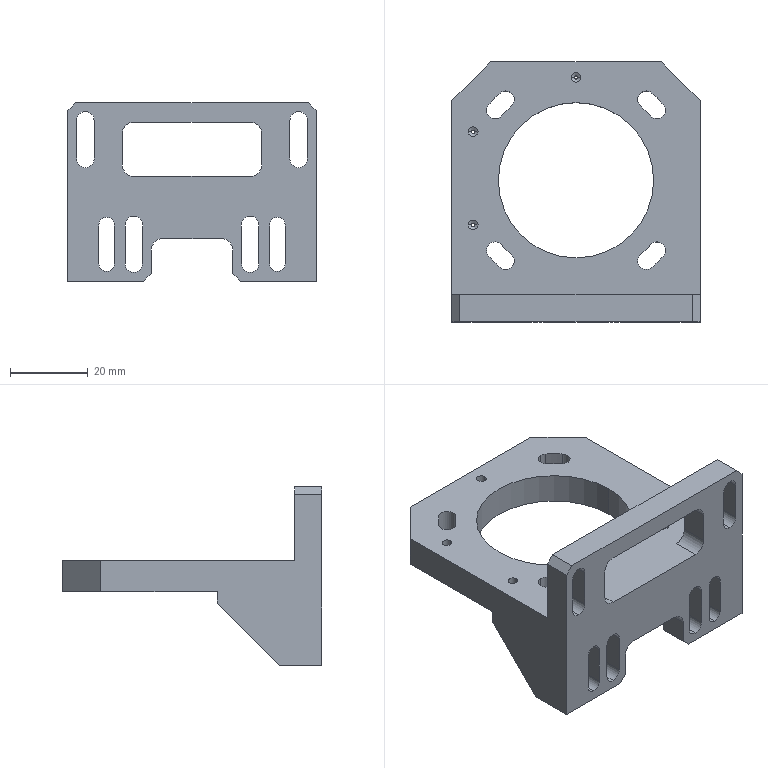NC program | NX | posted with a generic post | part box 64 x 67 x 46 mm
Lines 14041 to 14131 of 33790:
(DRILLING , TOOL : ZXZ)
N28068 T01 M6
N28070 G54
N28072 G17 G0 G90 X29.5 Y0. B0. C0. S3500 M3
N28074 G43 Z30. H1
N28076 G94 G81 G98 Z-20. F250. R-16.
N28078 X3.
N28080 X-8.5 Y26.5
N28082 X15.5
N28084 G80
N28086 G0 X15.5 Y26.5 Z30.
N28088 M5
(DRILLING_COPY , TOOL : 2.5ZT)
N28090 T12 M6
N28092 G54
N28094 G17 G0 G90 X29.5 Y0. B0. C0. S2000 M3
N28096 G43 Z30. H12
N28098 G94 G83 G98 Z-27.251 F120. Q2. R-16.
N28100 X15.5 Y26.5
N28102 X-8.5
N28104 G80
N28106 G0 X-8.5 Y26.5 Z30.
N28108 M5
(ZLEVEL_PROFILE_COPY , TOOL : D10JING)
N28110 T11 M6
N28112 G54
N28114 G17 G0 G90 X4.805 Y12.874 B0. C0. S5000 M3
N28116 G43 Z30. H11
N28118 Z-25.5
N28120 G94 G1 Z-27. F1000.
N28122 X3.866 Y14.5
N28124 G3 X3. Y15. R1.
N28126 X-12. Y0. R15. F1200.
N28128 X3. Y15. R-15.
N28130 X2.134 Y14.5 R1.
N28132 G1 X1.195 Y12.874
N28134 Z-25.5
N28136 G0 Z30.
(FLOOR_WALL_2 , TOOL : D10JING)
N28138 X34.03 Y29.956 S7000
N28140 Z-18.
N28142 G1 Z-19. F1250.
N28144 X33.999 Y29.938
N28146 G3 X33.499 Y29.072 R1.
N28148 G1 Y-29.072
N28150 X28.545 Y-34.027
N28152 Y34.027
N28154 X25.571 Y37.
N28156 X23.59
N28158 Y-37.
N28160 X18.636
N28162 Y37.
N28164 X13.681
N28166 Y-37.
N28168 X8.727
N28170 Y37.
N28172 X3.772
N28174 Y-37.
N28176 X-1.182
N28178 Y37.
N28180 X-6.137
N28182 Y-37.
N28184 X-11.091
N28186 Y37.
N28188 X-16.046
N28190 Y-37.
N28192 X-21.
N28194 Y37.
N28196 G2 X-20.5 Y37.866 R1.
N28198 G1 X-20.268 Y38.
N28200 Z-18.
N28202 G0 Z-15.9
N28204 X-20.768
N28206 Z-18.
N28208 G1 Z-19.
N28210 X-21. Y37.866
N28212 G3 X-21.5 Y37. R1.
N28214 G1 Y-37.
N28216 G3 X-21. Y-37.866 R1.
N28218 G1 X-20.768 Y-38.
N28220 Z-18.
N28222 G0 Z30.
N28224 M5